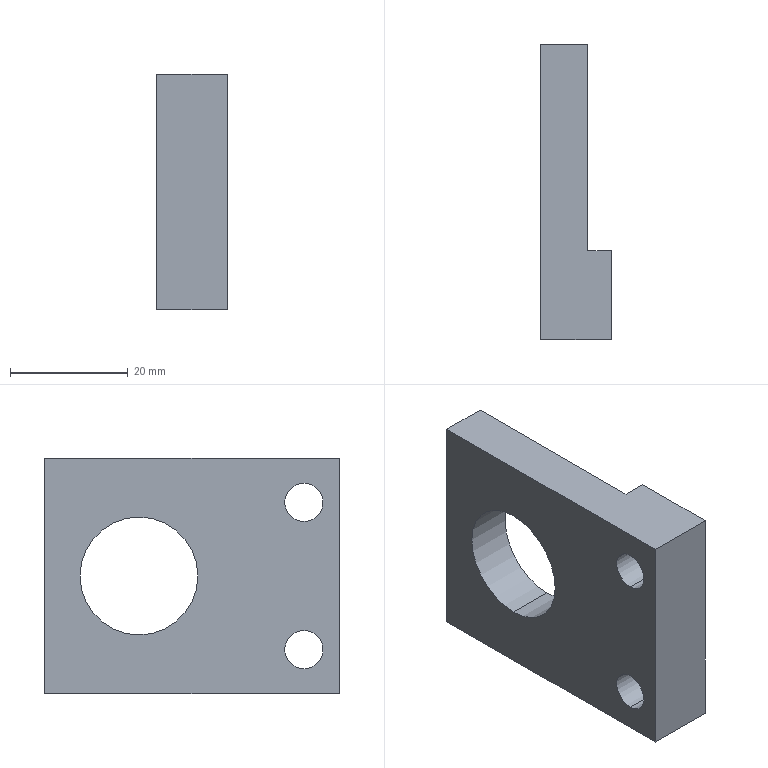Part | STEP file | cup material feed cylinder seat | 1 solid | 14 faces | box 12 x 50 x 40 mm | volume 15090 mm3 | plane 8 | cylinder 6 | commonest cylinder face diameters 6.5 x4 20 x2
STEP:
#1=CARTESIAN_POINT('',(0.,0.,0.));
#2=DIRECTION('',(0.,0.,1.));
#3=DIRECTION('',(1.,0.,0.));
#4=AXIS2_PLACEMENT_3D('',#1,#2,#3);
#5=CARTESIAN_POINT('',(0.,34.,-10.));
#6=VERTEX_POINT('',#5);
#7=CARTESIAN_POINT('',(8.,34.,-10.));
#8=VERTEX_POINT('',#7);
#9=CARTESIAN_POINT('',(8.,34.,-10.));
#10=DIRECTION('',(1.,0.,0.));
#11=VECTOR('',#10,1.);
#12=LINE('',#9,#11);
#13=CARTESIAN_POINT('',(8.,34.,0.));
#14=DIRECTION('',(1.,0.,0.));
#15=DIRECTION('',(0.,0.,-1.));
#16=AXIS2_PLACEMENT_3D('',#13,#14,#15);
#17=CYLINDRICAL_SURFACE('',#16,10.);
#18=CARTESIAN_POINT('',(6.283,0.));
#19=DIRECTION('',(0.,1.));
#20=VECTOR('',#19,1.);
#21=LINE('',#18,#20);
#22=(GEOMETRIC_REPRESENTATION_CONTEXT(2)PARAMETRIC_REPRESENTATION_CONTEXT()REPRESENTATION_CONTEXT('',''));
#23=DEFINITIONAL_REPRESENTATION('',(#21),#22);
#24=PCURVE('',#17,#23);
#25=CARTESIAN_POINT('',(8.,34.,0.));
#26=DIRECTION('',(1.,0.,0.));
#27=DIRECTION('',(0.,0.,-1.));
#28=AXIS2_PLACEMENT_3D('',#25,#26,#27);
#29=CYLINDRICAL_SURFACE('',#28,10.);
#30=CARTESIAN_POINT('',(0.,0.));
#31=DIRECTION('',(0.,1.));
#32=VECTOR('',#31,1.);
#33=LINE('',#30,#32);
#34=(GEOMETRIC_REPRESENTATION_CONTEXT(2)PARAMETRIC_REPRESENTATION_CONTEXT()REPRESENTATION_CONTEXT('',''));
#35=DEFINITIONAL_REPRESENTATION('',(#33),#34);
#36=PCURVE('',#29,#35);
#37=SURFACE_CURVE('',#12,(#24,#36),.PCURVE_S1.);
#38=EDGE_CURVE('',#6,#8,#37,.T.);
#39=ORIENTED_EDGE('',*,*,#38,.T.);
#40=CARTESIAN_POINT('',(8.,34.,10.));
#41=VERTEX_POINT('',#40);
#42=CARTESIAN_POINT('',(8.,34.,0.));
#43=DIRECTION('',(1.,0.,0.));
#44=DIRECTION('',(0.,0.,-1.));
#45=AXIS2_PLACEMENT_3D('',#42,#43,#44);
#46=CIRCLE('',#45,10.);
#47=CARTESIAN_POINT('',(0.,0.));
#48=DIRECTION('',(1.,0.));
#49=VECTOR('',#48,1.);
#50=LINE('',#47,#49);
#51=(GEOMETRIC_REPRESENTATION_CONTEXT(2)PARAMETRIC_REPRESENTATION_CONTEXT()REPRESENTATION_CONTEXT('',''));
#52=DEFINITIONAL_REPRESENTATION('',(#50),#51);
#53=PCURVE('',#17,#52);
#54=CARTESIAN_POINT('',(8.,50.,-20.));
#55=DIRECTION('',(1.,0.,0.));
#56=DIRECTION('',(0.,0.,-1.));
#57=AXIS2_PLACEMENT_3D('',#54,#55,#56);
#58=PLANE('',#57);
#59=CARTESIAN_POINT('',(-20.,-16.));
#60=DIRECTION('',(1.,0.));
#61=AXIS2_PLACEMENT_2D('',#59,#60);
#62=CIRCLE('',#61,10.);
#63=(GEOMETRIC_REPRESENTATION_CONTEXT(2)PARAMETRIC_REPRESENTATION_CONTEXT()REPRESENTATION_CONTEXT('',''));
#64=DEFINITIONAL_REPRESENTATION('',(#62),#63);
#65=PCURVE('',#58,#64);
#66=SURFACE_CURVE('',#46,(#53,#65),.PCURVE_S1.);
#67=EDGE_CURVE('',#41,#8,#66,.T.);
#68=ORIENTED_EDGE('',*,*,#67,.F.);
#69=CARTESIAN_POINT('',(0.,34.,10.));
#70=VERTEX_POINT('',#69);
#71=CARTESIAN_POINT('',(8.,34.,10.));
#72=DIRECTION('',(1.,0.,0.));
#73=VECTOR('',#72,1.);
#74=LINE('',#71,#73);
#75=CARTESIAN_POINT('',(3.142,0.));
#76=DIRECTION('',(0.,1.));
#77=VECTOR('',#76,1.);
#78=LINE('',#75,#77);
#79=(GEOMETRIC_REPRESENTATION_CONTEXT(2)PARAMETRIC_REPRESENTATION_CONTEXT()REPRESENTATION_CONTEXT('',''));
#80=DEFINITIONAL_REPRESENTATION('',(#78),#79);
#81=PCURVE('',#17,#80);
#82=CARTESIAN_POINT('',(3.142,0.));
#83=DIRECTION('',(0.,1.));
#84=VECTOR('',#83,1.);
#85=LINE('',#82,#84);
#86=(GEOMETRIC_REPRESENTATION_CONTEXT(2)PARAMETRIC_REPRESENTATION_CONTEXT()REPRESENTATION_CONTEXT('',''));
#87=DEFINITIONAL_REPRESENTATION('',(#85),#86);
#88=PCURVE('',#29,#87);
#89=SURFACE_CURVE('',#74,(#81,#88),.PCURVE_S1.);
#90=EDGE_CURVE('',#70,#41,#89,.T.);
#91=ORIENTED_EDGE('',*,*,#90,.F.);
#92=CARTESIAN_POINT('',(0.,34.,0.));
#93=DIRECTION('',(-1.,0.,0.));
#94=DIRECTION('',(0.,0.,1.));
#95=AXIS2_PLACEMENT_3D('',#92,#93,#94);
#96=CIRCLE('',#95,10.);
#97=CARTESIAN_POINT('',(9.425,-8.));
#98=DIRECTION('',(-1.,0.));
#99=VECTOR('',#98,1.);
#100=LINE('',#97,#99);
#101=(GEOMETRIC_REPRESENTATION_CONTEXT(2)PARAMETRIC_REPRESENTATION_CONTEXT()REPRESENTATION_CONTEXT('',''));
#102=DEFINITIONAL_REPRESENTATION('',(#100),#101);
#103=PCURVE('',#17,#102);
#104=CARTESIAN_POINT('',(0.,50.,-20.));
#105=DIRECTION('',(-1.,0.,0.));
#106=DIRECTION('',(0.,0.,1.));
#107=AXIS2_PLACEMENT_3D('',#104,#105,#106);
#108=PLANE('',#107);
#109=CARTESIAN_POINT('',(20.,-16.));
#110=DIRECTION('',(1.,0.));
#111=AXIS2_PLACEMENT_2D('',#109,#110);
#112=CIRCLE('',#111,10.);
#113=(GEOMETRIC_REPRESENTATION_CONTEXT(2)PARAMETRIC_REPRESENTATION_CONTEXT()REPRESENTATION_CONTEXT('',''));
#114=DEFINITIONAL_REPRESENTATION('',(#112),#113);
#115=PCURVE('',#108,#114);
#116=SURFACE_CURVE('',#96,(#103,#115),.PCURVE_S1.);
#117=EDGE_CURVE('',#6,#70,#116,.T.);
#118=ORIENTED_EDGE('',*,*,#117,.F.);
#119=EDGE_LOOP('',(#39,#68,#91,#118));
#120=FACE_BOUND('',#119,.F.);
#121=ADVANCED_FACE('',(#120),#17,.F.);
#122=CARTESIAN_POINT('',(0.,6.,9.25));
#123=VERTEX_POINT('',#122);
#124=CARTESIAN_POINT('',(12.,6.,9.25));
#125=VERTEX_POINT('',#124);
#126=CARTESIAN_POINT('',(12.,6.,9.25));
#127=DIRECTION('',(1.,0.,0.));
#128=VECTOR('',#127,1.);
#129=LINE('',#126,#128);
#130=CARTESIAN_POINT('',(12.,6.,12.5));
#131=DIRECTION('',(1.,0.,0.));
#132=DIRECTION('',(0.,0.,-1.));
#133=AXIS2_PLACEMENT_3D('',#130,#131,#132);
#134=CYLINDRICAL_SURFACE('',#133,3.25);
#135=CARTESIAN_POINT('',(6.283,0.));
#136=DIRECTION('',(0.,1.));
#137=VECTOR('',#136,1.);
#138=LINE('',#135,#137);
#139=(GEOMETRIC_REPRESENTATION_CONTEXT(2)PARAMETRIC_REPRESENTATION_CONTEXT()REPRESENTATION_CONTEXT('',''));
#140=DEFINITIONAL_REPRESENTATION('',(#138),#139);
#141=PCURVE('',#134,#140);
#142=CARTESIAN_POINT('',(12.,6.,12.5));
#143=DIRECTION('',(1.,0.,0.));
#144=DIRECTION('',(0.,0.,-1.));
#145=AXIS2_PLACEMENT_3D('',#142,#143,#144);
#146=CYLINDRICAL_SURFACE('',#145,3.25);
#147=CARTESIAN_POINT('',(0.,0.));
#148=DIRECTION('',(0.,1.));
#149=VECTOR('',#148,1.);
#150=LINE('',#147,#149);
#151=(GEOMETRIC_REPRESENTATION_CONTEXT(2)PARAMETRIC_REPRESENTATION_CONTEXT()REPRESENTATION_CONTEXT('',''));
#152=DEFINITIONAL_REPRESENTATION('',(#150),#151);
#153=PCURVE('',#146,#152);
#154=SURFACE_CURVE('',#129,(#141,#153),.PCURVE_S1.);
#155=EDGE_CURVE('',#123,#125,#154,.T.);
#156=ORIENTED_EDGE('',*,*,#155,.T.);
#157=CARTESIAN_POINT('',(12.,6.,15.75));
#158=VERTEX_POINT('',#157);
#159=CARTESIAN_POINT('',(12.,6.,12.5));
#160=DIRECTION('',(1.,0.,0.));
#161=DIRECTION('',(0.,0.,-1.));
#162=AXIS2_PLACEMENT_3D('',#159,#160,#161);
#163=CIRCLE('',#162,3.25);
#164=CARTESIAN_POINT('',(0.,0.));
#165=DIRECTION('',(1.,0.));
#166=VECTOR('',#165,1.);
#167=LINE('',#164,#166);
#168=(GEOMETRIC_REPRESENTATION_CONTEXT(2)PARAMETRIC_REPRESENTATION_CONTEXT()REPRESENTATION_CONTEXT('',''));
#169=DEFINITIONAL_REPRESENTATION('',(#167),#168);
#170=PCURVE('',#134,#169);
#171=CARTESIAN_POINT('',(12.,15.,-20.));
#172=DIRECTION('',(1.,0.,0.));
#173=DIRECTION('',(0.,0.,-1.));
#174=AXIS2_PLACEMENT_3D('',#171,#172,#173);
#175=PLANE('',#174);
#176=CARTESIAN_POINT('',(-32.5,-9.));
#177=DIRECTION('',(1.,0.));
#178=AXIS2_PLACEMENT_2D('',#176,#177);
#179=CIRCLE('',#178,3.25);
#180=(GEOMETRIC_REPRESENTATION_CONTEXT(2)PARAMETRIC_REPRESENTATION_CONTEXT()REPRESENTATION_CONTEXT('',''));
#181=DEFINITIONAL_REPRESENTATION('',(#179),#180);
#182=PCURVE('',#175,#181);
#183=SURFACE_CURVE('',#163,(#170,#182),.PCURVE_S1.);
#184=EDGE_CURVE('',#158,#125,#183,.T.);
#185=ORIENTED_EDGE('',*,*,#184,.F.);
#186=CARTESIAN_POINT('',(0.,6.,15.75));
#187=VERTEX_POINT('',#186);
#188=CARTESIAN_POINT('',(12.,6.,15.75));
#189=DIRECTION('',(1.,0.,0.));
#190=VECTOR('',#189,1.);
#191=LINE('',#188,#190);
#192=CARTESIAN_POINT('',(3.142,0.));
#193=DIRECTION('',(0.,1.));
#194=VECTOR('',#193,1.);
#195=LINE('',#192,#194);
#196=(GEOMETRIC_REPRESENTATION_CONTEXT(2)PARAMETRIC_REPRESENTATION_CONTEXT()REPRESENTATION_CONTEXT('',''));
#197=DEFINITIONAL_REPRESENTATION('',(#195),#196);
#198=PCURVE('',#134,#197);
#199=CARTESIAN_POINT('',(3.142,0.));
#200=DIRECTION('',(0.,1.));
#201=VECTOR('',#200,1.);
#202=LINE('',#199,#201);
#203=(GEOMETRIC_REPRESENTATION_CONTEXT(2)PARAMETRIC_REPRESENTATION_CONTEXT()REPRESENTATION_CONTEXT('',''));
#204=DEFINITIONAL_REPRESENTATION('',(#202),#203);
#205=PCURVE('',#146,#204);
#206=SURFACE_CURVE('',#191,(#198,#205),.PCURVE_S1.);
#207=EDGE_CURVE('',#187,#158,#206,.T.);
#208=ORIENTED_EDGE('',*,*,#207,.F.);
#209=CARTESIAN_POINT('',(0.,6.,12.5));
#210=DIRECTION('',(1.,0.,0.));
#211=DIRECTION('',(0.,0.,-1.));
#212=AXIS2_PLACEMENT_3D('',#209,#210,#211);
#213=CIRCLE('',#212,3.25);
#214=CARTESIAN_POINT('',(0.,-12.));
#215=DIRECTION('',(1.,0.));
#216=VECTOR('',#215,1.);
#217=LINE('',#214,#216);
#218=(GEOMETRIC_REPRESENTATION_CONTEXT(2)PARAMETRIC_REPRESENTATION_CONTEXT()REPRESENTATION_CONTEXT('',''));
#219=DEFINITIONAL_REPRESENTATION('',(#217),#218);
#220=PCURVE('',#134,#219);
#221=CARTESIAN_POINT('',(29.25,-44.));
#222=CARTESIAN_POINT('',(29.25,-38.371));
#223=CARTESIAN_POINT('',(34.125,-41.185));
#224=CARTESIAN_POINT('',(39.,-44.));
#225=CARTESIAN_POINT('',(34.125,-46.815));
#226=CARTESIAN_POINT('',(29.25,-49.629));
#227=CARTESIAN_POINT('',(29.25,-44.));
#228=(BOUNDED_CURVE()B_SPLINE_CURVE(2,(#221,#222,#223,#224,#225,#226,#227),.UNSPECIFIED.,.T.,.F.)B_SPLINE_CURVE_WITH_KNOTS((1,2,2,2,2,1),(-2.094,0.,2.094,4.189,6.283,8.378),.UNSPECIFIED.)CURVE()GEOMETRIC_REPRESENTATION_ITEM()RATIONAL_B_SPLINE_CURVE((1.,0.5,1.,0.5,1.,0.5,1.))REPRESENTATION_ITEM(''));
#229=(GEOMETRIC_REPRESENTATION_CONTEXT(2)PARAMETRIC_REPRESENTATION_CONTEXT()REPRESENTATION_CONTEXT('',''));
#230=DEFINITIONAL_REPRESENTATION('',(#228),#229);
#231=PCURVE('',#108,#230);
#232=SURFACE_CURVE('',#213,(#220,#231),.PCURVE_S1.);
#233=EDGE_CURVE('',#187,#123,#232,.T.);
#234=ORIENTED_EDGE('',*,*,#233,.T.);
#235=EDGE_LOOP('',(#156,#185,#208,#234));
#236=FACE_BOUND('',#235,.F.);
#237=ADVANCED_FACE('',(#236),#134,.F.);
#238=CARTESIAN_POINT('',(0.,6.,-15.75));
#239=VERTEX_POINT('',#238);
#240=CARTESIAN_POINT('',(12.,6.,-15.75));
#241=VERTEX_POINT('',#240);
#242=CARTESIAN_POINT('',(12.,6.,-15.75));
#243=DIRECTION('',(1.,0.,0.));
#244=VECTOR('',#243,1.);
#245=LINE('',#242,#244);
#246=CARTESIAN_POINT('',(12.,6.,-12.5));
#247=DIRECTION('',(1.,0.,0.));
#248=DIRECTION('',(0.,0.,-1.));
#249=AXIS2_PLACEMENT_3D('',#246,#247,#248);
#250=CYLINDRICAL_SURFACE('',#249,3.25);
#251=CARTESIAN_POINT('',(6.283,0.));
#252=DIRECTION('',(0.,1.));
#253=VECTOR('',#252,1.);
#254=LINE('',#251,#253);
#255=(GEOMETRIC_REPRESENTATION_CONTEXT(2)PARAMETRIC_REPRESENTATION_CONTEXT()REPRESENTATION_CONTEXT('',''));
#256=DEFINITIONAL_REPRESENTATION('',(#254),#255);
#257=PCURVE('',#250,#256);
#258=CARTESIAN_POINT('',(12.,6.,-12.5));
#259=DIRECTION('',(1.,0.,0.));
#260=DIRECTION('',(0.,0.,-1.));
#261=AXIS2_PLACEMENT_3D('',#258,#259,#260);
#262=CYLINDRICAL_SURFACE('',#261,3.25);
#263=CARTESIAN_POINT('',(0.,0.));
#264=DIRECTION('',(0.,1.));
#265=VECTOR('',#264,1.);
#266=LINE('',#263,#265);
#267=(GEOMETRIC_REPRESENTATION_CONTEXT(2)PARAMETRIC_REPRESENTATION_CONTEXT()REPRESENTATION_CONTEXT('',''));
#268=DEFINITIONAL_REPRESENTATION('',(#266),#267);
#269=PCURVE('',#262,#268);
#270=SURFACE_CURVE('',#245,(#257,#269),.PCURVE_S1.);
#271=EDGE_CURVE('',#239,#241,#270,.T.);
#272=ORIENTED_EDGE('',*,*,#271,.T.);
#273=CARTESIAN_POINT('',(12.,6.,-9.25));
#274=VERTEX_POINT('',#273);
#275=CARTESIAN_POINT('',(12.,6.,-12.5));
#276=DIRECTION('',(1.,0.,0.));
#277=DIRECTION('',(0.,0.,-1.));
#278=AXIS2_PLACEMENT_3D('',#275,#276,#277);
#279=CIRCLE('',#278,3.25);
#280=CARTESIAN_POINT('',(0.,0.));
#281=DIRECTION('',(1.,0.));
#282=VECTOR('',#281,1.);
#283=LINE('',#280,#282);
#284=(GEOMETRIC_REPRESENTATION_CONTEXT(2)PARAMETRIC_REPRESENTATION_CONTEXT()REPRESENTATION_CONTEXT('',''));
#285=DEFINITIONAL_REPRESENTATION('',(#283),#284);
#286=PCURVE('',#250,#285);
#287=CARTESIAN_POINT('',(-7.5,-9.));
#288=DIRECTION('',(1.,0.));
#289=AXIS2_PLACEMENT_2D('',#287,#288);
#290=CIRCLE('',#289,3.25);
#291=(GEOMETRIC_REPRESENTATION_CONTEXT(2)PARAMETRIC_REPRESENTATION_CONTEXT()REPRESENTATION_CONTEXT('',''));
#292=DEFINITIONAL_REPRESENTATION('',(#290),#291);
#293=PCURVE('',#175,#292);
#294=SURFACE_CURVE('',#279,(#286,#293),.PCURVE_S1.);
#295=EDGE_CURVE('',#274,#241,#294,.T.);
#296=ORIENTED_EDGE('',*,*,#295,.F.);
#297=CARTESIAN_POINT('',(0.,6.,-9.25));
#298=VERTEX_POINT('',#297);
#299=CARTESIAN_POINT('',(12.,6.,-9.25));
#300=DIRECTION('',(1.,0.,0.));
#301=VECTOR('',#300,1.);
#302=LINE('',#299,#301);
#303=CARTESIAN_POINT('',(3.142,0.));
#304=DIRECTION('',(0.,1.));
#305=VECTOR('',#304,1.);
#306=LINE('',#303,#305);
#307=(GEOMETRIC_REPRESENTATION_CONTEXT(2)PARAMETRIC_REPRESENTATION_CONTEXT()REPRESENTATION_CONTEXT('',''));
#308=DEFINITIONAL_REPRESENTATION('',(#306),#307);
#309=PCURVE('',#250,#308);
#310=CARTESIAN_POINT('',(3.142,0.));
#311=DIRECTION('',(0.,1.));
#312=VECTOR('',#311,1.);
#313=LINE('',#310,#312);
#314=(GEOMETRIC_REPRESENTATION_CONTEXT(2)PARAMETRIC_REPRESENTATION_CONTEXT()REPRESENTATION_CONTEXT('',''));
#315=DEFINITIONAL_REPRESENTATION('',(#313),#314);
#316=PCURVE('',#262,#315);
#317=SURFACE_CURVE('',#302,(#309,#316),.PCURVE_S1.);
#318=EDGE_CURVE('',#298,#274,#317,.T.);
#319=ORIENTED_EDGE('',*,*,#318,.F.);
#320=CARTESIAN_POINT('',(0.,6.,-12.5));
#321=DIRECTION('',(1.,0.,0.));
#322=DIRECTION('',(0.,0.,-1.));
#323=AXIS2_PLACEMENT_3D('',#320,#321,#322);
#324=CIRCLE('',#323,3.25);
#325=CARTESIAN_POINT('',(0.,-12.));
#326=DIRECTION('',(1.,0.));
#327=VECTOR('',#326,1.);
#328=LINE('',#325,#327);
#329=(GEOMETRIC_REPRESENTATION_CONTEXT(2)PARAMETRIC_REPRESENTATION_CONTEXT()REPRESENTATION_CONTEXT('',''));
#330=DEFINITIONAL_REPRESENTATION('',(#328),#329);
#331=PCURVE('',#250,#330);
#332=CARTESIAN_POINT('',(4.25,-44.));
#333=CARTESIAN_POINT('',(4.25,-38.371));
#334=CARTESIAN_POINT('',(9.125,-41.185));
#335=CARTESIAN_POINT('',(14.,-44.));
#336=CARTESIAN_POINT('',(9.125,-46.815));
#337=CARTESIAN_POINT('',(4.25,-49.629));
#338=CARTESIAN_POINT('',(4.25,-44.));
#339=(BOUNDED_CURVE()B_SPLINE_CURVE(2,(#332,#333,#334,#335,#336,#337,#338),.UNSPECIFIED.,.T.,.F.)B_SPLINE_CURVE_WITH_KNOTS((1,2,2,2,2,1),(-2.094,0.,2.094,4.189,6.283,8.378),.UNSPECIFIED.)CURVE()GEOMETRIC_REPRESENTATION_ITEM()RATIONAL_B_SPLINE_CURVE((1.,0.5,1.,0.5,1.,0.5,1.))REPRESENTATION_ITEM(''));
#340=(GEOMETRIC_REPRESENTATION_CONTEXT(2)PARAMETRIC_REPRESENTATION_CONTEXT()REPRESENTATION_CONTEXT('',''));
#341=DEFINITIONAL_REPRESENTATION('',(#339),#340);
#342=PCURVE('',#108,#341);
#343=SURFACE_CURVE('',#324,(#331,#342),.PCURVE_S1.);
#344=EDGE_CURVE('',#298,#239,#343,.T.);
#345=ORIENTED_EDGE('',*,*,#344,.T.);
#346=EDGE_LOOP('',(#272,#296,#319,#345));
#347=FACE_BOUND('',#346,.F.);
#348=ADVANCED_FACE('',(#347),#250,.F.);
#349=ORIENTED_EDGE('',*,*,#117,.F.);
#350=CARTESIAN_POINT('',(0.,34.,0.));
#351=DIRECTION('',(-1.,0.,0.));
#352=DIRECTION('',(0.,0.,1.));
#353=AXIS2_PLACEMENT_3D('',#350,#351,#352);
#354=CIRCLE('',#353,10.);
#355=CARTESIAN_POINT('',(20.,-16.));
#356=DIRECTION('',(1.,0.));
#357=AXIS2_PLACEMENT_2D('',#355,#356);
#358=CIRCLE('',#357,10.);
#359=(GEOMETRIC_REPRESENTATION_CONTEXT(2)PARAMETRIC_REPRESENTATION_CONTEXT()REPRESENTATION_CONTEXT('',''));
#360=DEFINITIONAL_REPRESENTATION('',(#358),#359);
#361=PCURVE('',#108,#360);
#362=CARTESIAN_POINT('',(3.142,-8.));
#363=DIRECTION('',(-1.,0.));
#364=VECTOR('',#363,1.);
#365=LINE('',#362,#364);
#366=(GEOMETRIC_REPRESENTATION_CONTEXT(2)PARAMETRIC_REPRESENTATION_CONTEXT()REPRESENTATION_CONTEXT('',''));
#367=DEFINITIONAL_REPRESENTATION('',(#365),#366);
#368=PCURVE('',#29,#367);
#369=SURFACE_CURVE('',#354,(#361,#368),.PCURVE_S1.);
#370=EDGE_CURVE('',#70,#6,#369,.T.);
#371=ORIENTED_EDGE('',*,*,#370,.F.);
#372=EDGE_LOOP('',(#349,#371));
#373=FACE_BOUND('',#372,.T.);
#374=CARTESIAN_POINT('',(0.,6.,12.5));
#375=DIRECTION('',(1.,0.,0.));
#376=DIRECTION('',(0.,0.,-1.));
#377=AXIS2_PLACEMENT_3D('',#374,#375,#376);
#378=CIRCLE('',#377,3.25);
#379=CARTESIAN_POINT('',(29.25,-44.));
#380=CARTESIAN_POINT('',(29.25,-38.371));
#381=CARTESIAN_POINT('',(34.125,-41.185));
#382=CARTESIAN_POINT('',(39.,-44.));
#383=CARTESIAN_POINT('',(34.125,-46.815));
#384=CARTESIAN_POINT('',(29.25,-49.629));
#385=CARTESIAN_POINT('',(29.25,-44.));
#386=(BOUNDED_CURVE()B_SPLINE_CURVE(2,(#379,#380,#381,#382,#383,#384,#385),.UNSPECIFIED.,.T.,.F.)B_SPLINE_CURVE_WITH_KNOTS((1,2,2,2,2,1),(-2.094,0.,2.094,4.189,6.283,8.378),.UNSPECIFIED.)CURVE()GEOMETRIC_REPRESENTATION_ITEM()RATIONAL_B_SPLINE_CURVE((1.,0.5,1.,0.5,1.,0.5,1.))REPRESENTATION_ITEM(''));
#387=(GEOMETRIC_REPRESENTATION_CONTEXT(2)PARAMETRIC_REPRESENTATION_CONTEXT()REPRESENTATION_CONTEXT('',''));
#388=DEFINITIONAL_REPRESENTATION('',(#386),#387);
#389=PCURVE('',#108,#388);
#390=CARTESIAN_POINT('',(0.,-12.));
#391=DIRECTION('',(1.,0.));
#392=VECTOR('',#391,1.);
#393=LINE('',#390,#392);
#394=(GEOMETRIC_REPRESENTATION_CONTEXT(2)PARAMETRIC_REPRESENTATION_CONTEXT()REPRESENTATION_CONTEXT('',''));
#395=DEFINITIONAL_REPRESENTATION('',(#393),#394);
#396=PCURVE('',#146,#395);
#397=SURFACE_CURVE('',#378,(#389,#396),.PCURVE_S1.);
#398=EDGE_CURVE('',#123,#187,#397,.T.);
#399=ORIENTED_EDGE('',*,*,#398,.T.);
#400=ORIENTED_EDGE('',*,*,#233,.T.);
#401=EDGE_LOOP('',(#399,#400));
#402=FACE_BOUND('',#401,.T.);
#403=CARTESIAN_POINT('',(0.,6.,-12.5));
#404=DIRECTION('',(1.,0.,0.));
#405=DIRECTION('',(0.,0.,-1.));
#406=AXIS2_PLACEMENT_3D('',#403,#404,#405);
#407=CIRCLE('',#406,3.25);
#408=CARTESIAN_POINT('',(4.25,-44.));
#409=CARTESIAN_POINT('',(4.25,-38.371));
#410=CARTESIAN_POINT('',(9.125,-41.185));
#411=CARTESIAN_POINT('',(14.,-44.));
#412=CARTESIAN_POINT('',(9.125,-46.815));
#413=CARTESIAN_POINT('',(4.25,-49.629));
#414=CARTESIAN_POINT('',(4.25,-44.));
#415=(BOUNDED_CURVE()B_SPLINE_CURVE(2,(#408,#409,#410,#411,#412,#413,#414),.UNSPECIFIED.,.T.,.F.)B_SPLINE_CURVE_WITH_KNOTS((1,2,2,2,2,1),(-2.094,0.,2.094,4.189,6.283,8.378),.UNSPECIFIED.)CURVE()GEOMETRIC_REPRESENTATION_ITEM()RATIONAL_B_SPLINE_CURVE((1.,0.5,1.,0.5,1.,0.5,1.))REPRESENTATION_ITEM(''));
#416=(GEOMETRIC_REPRESENTATION_CONTEXT(2)PARAMETRIC_REPRESENTATION_CONTEXT()REPRESENTATION_CONTEXT('',''));
#417=DEFINITIONAL_REPRESENTATION('',(#415),#416);
#418=PCURVE('',#108,#417);
#419=CARTESIAN_POINT('',(0.,-12.));
#420=DIRECTION('',(1.,0.));
#421=VECTOR('',#420,1.);
#422=LINE('',#419,#421);
#423=(GEOMETRIC_REPRESENTATION_CONTEXT(2)PARAMETRIC_REPRESENTATION_CONTEXT()REPRESENTATION_CONTEXT('',''));
#424=DEFINITIONAL_REPRESENTATION('',(#422),#423);
#425=PCURVE('',#262,#424);
#426=SURFACE_CURVE('',#407,(#418,#425),.PCURVE_S1.);
#427=EDGE_CURVE('',#239,#298,#426,.T.);
#428=ORIENTED_EDGE('',*,*,#427,.T.);
#429=ORIENTED_EDGE('',*,*,#344,.T.);
#430=EDGE_LOOP('',(#428,#429));
#431=FACE_BOUND('',#430,.T.);
#432=CARTESIAN_POINT('',(0.,0.,-20.));
#433=VERTEX_POINT('',#432);
#434=CARTESIAN_POINT('',(0.,0.,20.));
#435=VERTEX_POINT('',#434);
#436=CARTESIAN_POINT('',(0.,0.,-20.));
#437=DIRECTION('',(0.,0.,1.));
#438=VECTOR('',#437,1.);
#439=LINE('',#436,#438);
#440=CARTESIAN_POINT('',(0.,-50.));
#441=DIRECTION('',(1.,0.));
#442=VECTOR('',#441,1.);
#443=LINE('',#440,#442);
#444=(GEOMETRIC_REPRESENTATION_CONTEXT(2)PARAMETRIC_REPRESENTATION_CONTEXT()REPRESENTATION_CONTEXT('',''));
#445=DEFINITIONAL_REPRESENTATION('',(#443),#444);
#446=PCURVE('',#108,#445);
#447=CARTESIAN_POINT('',(0.,0.,-20.));
#448=DIRECTION('',(0.,-1.,0.));
#449=DIRECTION('',(0.,0.,-1.));
#450=AXIS2_PLACEMENT_3D('',#447,#448,#449);
#451=PLANE('',#450);
#452=CARTESIAN_POINT('',(0.,0.));
#453=DIRECTION('',(-1.,0.));
#454=VECTOR('',#453,1.);
#455=LINE('',#452,#454);
#456=(GEOMETRIC_REPRESENTATION_CONTEXT(2)PARAMETRIC_REPRESENTATION_CONTEXT()REPRESENTATION_CONTEXT('',''));
#457=DEFINITIONAL_REPRESENTATION('',(#455),#456);
#458=PCURVE('',#451,#457);
#459=SURFACE_CURVE('',#439,(#446,#458),.PCURVE_S1.);
#460=EDGE_CURVE('',#433,#435,#459,.T.);
#461=ORIENTED_EDGE('',*,*,#460,.T.);
#462=CARTESIAN_POINT('',(0.,50.,20.));
#463=VERTEX_POINT('',#462);
#464=CARTESIAN_POINT('',(0.,50.,20.));
#465=DIRECTION('',(0.,-1.,0.));
#466=VECTOR('',#465,1.);
#467=LINE('',#464,#466);
#468=CARTESIAN_POINT('',(40.,0.));
#469=DIRECTION('',(0.,-1.));
#470=VECTOR('',#469,1.);
#471=LINE('',#468,#470);
#472=(GEOMETRIC_REPRESENTATION_CONTEXT(2)PARAMETRIC_REPRESENTATION_CONTEXT()REPRESENTATION_CONTEXT('',''));
#473=DEFINITIONAL_REPRESENTATION('',(#471),#472);
#474=PCURVE('',#108,#473);
#475=CARTESIAN_POINT('',(0.,0.,20.));
#476=DIRECTION('',(0.,0.,1.));
#477=DIRECTION('',(1.,0.,0.));
#478=AXIS2_PLACEMENT_3D('',#475,#476,#477);
#479=PLANE('',#478);
#480=CARTESIAN_POINT('',(0.,50.));
#481=DIRECTION('',(0.,-1.));
#482=VECTOR('',#481,1.);
#483=LINE('',#480,#482);
#484=(GEOMETRIC_REPRESENTATION_CONTEXT(2)PARAMETRIC_REPRESENTATION_CONTEXT()REPRESENTATION_CONTEXT('',''));
#485=DEFINITIONAL_REPRESENTATION('',(#483),#484);
#486=PCURVE('',#479,#485);
#487=SURFACE_CURVE('',#467,(#474,#486),.PCURVE_S1.);
#488=EDGE_CURVE('',#463,#435,#487,.T.);
#489=ORIENTED_EDGE('',*,*,#488,.F.);
#490=CARTESIAN_POINT('',(0.,50.,-20.));
#491=VERTEX_POINT('',#490);
#492=CARTESIAN_POINT('',(0.,50.,-20.));
#493=DIRECTION('',(0.,0.,1.));
#494=VECTOR('',#493,1.);
#495=LINE('',#492,#494);
#496=CARTESIAN_POINT('',(0.,0.));
#497=DIRECTION('',(1.,0.));
#498=VECTOR('',#497,1.);
#499=LINE('',#496,#498);
#500=(GEOMETRIC_REPRESENTATION_CONTEXT(2)PARAMETRIC_REPRESENTATION_CONTEXT()REPRESENTATION_CONTEXT('',''));
#501=DEFINITIONAL_REPRESENTATION('',(#499),#500);
#502=PCURVE('',#108,#501);
#503=CARTESIAN_POINT('',(0.,50.,-20.));
#504=DIRECTION('',(0.,1.,0.));
#505=DIRECTION('',(0.,0.,1.));
#506=AXIS2_PLACEMENT_3D('',#503,#504,#505);
#507=PLANE('',#506);
#508=CARTESIAN_POINT('',(0.,0.));
#509=DIRECTION('',(1.,0.));
#510=VECTOR('',#509,1.);
#511=LINE('',#508,#510);
#512=(GEOMETRIC_REPRESENTATION_CONTEXT(2)PARAMETRIC_REPRESENTATION_CONTEXT()REPRESENTATION_CONTEXT('',''));
#513=DEFINITIONAL_REPRESENTATION('',(#511),#512);
#514=PCURVE('',#507,#513);
#515=SURFACE_CURVE('',#495,(#502,#514),.PCURVE_S1.);
#516=EDGE_CURVE('',#491,#463,#515,.T.);
#517=ORIENTED_EDGE('',*,*,#516,.F.);
#518=CARTESIAN_POINT('',(0.,50.,-20.));
#519=DIRECTION('',(0.,-1.,0.));
#520=VECTOR('',#519,1.);
#521=LINE('',#518,#520);
#522=CARTESIAN_POINT('',(0.,0.));
#523=DIRECTION('',(0.,-1.));
#524=VECTOR('',#523,1.);
#525=LINE('',#522,#524);
#526=(GEOMETRIC_REPRESENTATION_CONTEXT(2)PARAMETRIC_REPRESENTATION_CONTEXT()REPRESENTATION_CONTEXT('',''));
#527=DEFINITIONAL_REPRESENTATION('',(#525),#526);
#528=PCURVE('',#108,#527);
#529=CARTESIAN_POINT('',(0.,0.,-20.));
#530=DIRECTION('',(0.,0.,1.));
#531=DIRECTION('',(1.,0.,0.));
#532=AXIS2_PLACEMENT_3D('',#529,#530,#531);
#533=PLANE('',#532);
#534=CARTESIAN_POINT('',(0.,50.));
#535=DIRECTION('',(0.,-1.));
#536=VECTOR('',#535,1.);
#537=LINE('',#534,#536);
#538=(GEOMETRIC_REPRESENTATION_CONTEXT(2)PARAMETRIC_REPRESENTATION_CONTEXT()REPRESENTATION_CONTEXT('',''));
#539=DEFINITIONAL_REPRESENTATION('',(#537),#538);
#540=PCURVE('',#533,#539);
#541=SURFACE_CURVE('',#521,(#528,#540),.PCURVE_S1.);
#542=EDGE_CURVE('',#491,#433,#541,.T.);
#543=ORIENTED_EDGE('',*,*,#542,.T.);
#544=EDGE_LOOP('',(#461,#489,#517,#543));
#545=FACE_BOUND('',#544,.T.);
#546=ADVANCED_FACE('',(#373,#402,#431,#545),#108,.T.);
#547=ORIENTED_EDGE('',*,*,#516,.T.);
#548=CARTESIAN_POINT('',(8.,50.,20.));
#549=VERTEX_POINT('',#548);
#550=CARTESIAN_POINT('',(0.,50.,20.));
#551=DIRECTION('',(-1.,0.,0.));
#552=VECTOR('',#551,1.);
#553=LINE('',#550,#552);
#554=CARTESIAN_POINT('',(40.,0.));
#555=DIRECTION('',(0.,-1.));
#556=VECTOR('',#555,1.);
#557=LINE('',#554,#556);
#558=(GEOMETRIC_REPRESENTATION_CONTEXT(2)PARAMETRIC_REPRESENTATION_CONTEXT()REPRESENTATION_CONTEXT('',''));
#559=DEFINITIONAL_REPRESENTATION('',(#557),#558);
#560=PCURVE('',#507,#559);
#561=CARTESIAN_POINT('',(0.,50.));
#562=DIRECTION('',(-1.,0.));
#563=VECTOR('',#562,1.);
#564=LINE('',#561,#563);
#565=(GEOMETRIC_REPRESENTATION_CONTEXT(2)PARAMETRIC_REPRESENTATION_CONTEXT()REPRESENTATION_CONTEXT('',''));
#566=DEFINITIONAL_REPRESENTATION('',(#564),#565);
#567=PCURVE('',#479,#566);
#568=SURFACE_CURVE('',#553,(#560,#567),.PCURVE_S1.);
#569=EDGE_CURVE('',#549,#463,#568,.T.);
#570=ORIENTED_EDGE('',*,*,#569,.F.);
#571=CARTESIAN_POINT('',(8.,50.,-20.));
#572=VERTEX_POINT('',#571);
#573=CARTESIAN_POINT('',(8.,50.,-20.));
#574=DIRECTION('',(0.,0.,1.));
#575=VECTOR('',#574,1.);
#576=LINE('',#573,#575);
#577=CARTESIAN_POINT('',(0.,8.));
#578=DIRECTION('',(1.,0.));
#579=VECTOR('',#578,1.);
#580=LINE('',#577,#579);
#581=(GEOMETRIC_REPRESENTATION_CONTEXT(2)PARAMETRIC_REPRESENTATION_CONTEXT()REPRESENTATION_CONTEXT('',''));
#582=DEFINITIONAL_REPRESENTATION('',(#580),#581);
#583=PCURVE('',#507,#582);
#584=CARTESIAN_POINT('',(0.,0.));
#585=DIRECTION('',(-1.,0.));
#586=VECTOR('',#585,1.);
#587=LINE('',#584,#586);
#588=(GEOMETRIC_REPRESENTATION_CONTEXT(2)PARAMETRIC_REPRESENTATION_CONTEXT()REPRESENTATION_CONTEXT('',''));
#589=DEFINITIONAL_REPRESENTATION('',(#587),#588);
#590=PCURVE('',#58,#589);
#591=SURFACE_CURVE('',#576,(#583,#590),.PCURVE_S1.);
#592=EDGE_CURVE('',#572,#549,#591,.T.);
#593=ORIENTED_EDGE('',*,*,#592,.F.);
#594=CARTESIAN_POINT('',(0.,50.,-20.));
#595=DIRECTION('',(-1.,0.,0.));
#596=VECTOR('',#595,1.);
#597=LINE('',#594,#596);
#598=CARTESIAN_POINT('',(0.,0.));
#599=DIRECTION('',(0.,-1.));
#600=VECTOR('',#599,1.);
#601=LINE('',#598,#600);
#602=(GEOMETRIC_REPRESENTATION_CONTEXT(2)PARAMETRIC_REPRESENTATION_CONTEXT()REPRESENTATION_CONTEXT('',''));
#603=DEFINITIONAL_REPRESENTATION('',(#601),#602);
#604=PCURVE('',#507,#603);
#605=CARTESIAN_POINT('',(0.,50.));
#606=DIRECTION('',(-1.,0.));
#607=VECTOR('',#606,1.);
#608=LINE('',#605,#607);
#609=(GEOMETRIC_REPRESENTATION_CONTEXT(2)PARAMETRIC_REPRESENTATION_CONTEXT()REPRESENTATION_CONTEXT('',''));
#610=DEFINITIONAL_REPRESENTATION('',(#608),#609);
#611=PCURVE('',#533,#610);
#612=SURFACE_CURVE('',#597,(#604,#611),.PCURVE_S1.);
#613=EDGE_CURVE('',#572,#491,#612,.T.);
#614=ORIENTED_EDGE('',*,*,#613,.T.);
#615=EDGE_LOOP('',(#547,#570,#593,#614));
#616=FACE_BOUND('',#615,.T.);
#617=ADVANCED_FACE('',(#616),#507,.T.);
#618=CARTESIAN_POINT('',(8.,34.,0.));
#619=DIRECTION('',(1.,0.,0.));
#620=DIRECTION('',(0.,0.,-1.));
#621=AXIS2_PLACEMENT_3D('',#618,#619,#620);
#622=CIRCLE('',#621,10.);
#623=CARTESIAN_POINT('',(-20.,-16.));
#624=DIRECTION('',(1.,0.));
#625=AXIS2_PLACEMENT_2D('',#623,#624);
#626=CIRCLE('',#625,10.);
#627=(GEOMETRIC_REPRESENTATION_CONTEXT(2)PARAMETRIC_REPRESENTATION_CONTEXT()REPRESENTATION_CONTEXT('',''));
#628=DEFINITIONAL_REPRESENTATION('',(#626),#627);
#629=PCURVE('',#58,#628);
#630=CARTESIAN_POINT('',(0.,0.));
#631=DIRECTION('',(1.,0.));
#632=VECTOR('',#631,1.);
#633=LINE('',#630,#632);
#634=(GEOMETRIC_REPRESENTATION_CONTEXT(2)PARAMETRIC_REPRESENTATION_CONTEXT()REPRESENTATION_CONTEXT('',''));
#635=DEFINITIONAL_REPRESENTATION('',(#633),#634);
#636=PCURVE('',#29,#635);
#637=SURFACE_CURVE('',#622,(#629,#636),.PCURVE_S1.);
#638=EDGE_CURVE('',#8,#41,#637,.T.);
#639=ORIENTED_EDGE('',*,*,#638,.F.);
#640=ORIENTED_EDGE('',*,*,#67,.F.);
#641=EDGE_LOOP('',(#639,#640));
#642=FACE_BOUND('',#641,.T.);
#643=ORIENTED_EDGE('',*,*,#592,.T.);
#644=CARTESIAN_POINT('',(8.,15.,20.));
#645=VERTEX_POINT('',#644);
#646=CARTESIAN_POINT('',(8.,50.,20.));
#647=DIRECTION('',(0.,1.,0.));
#648=VECTOR('',#647,1.);
#649=LINE('',#646,#648);
#650=CARTESIAN_POINT('',(-40.,0.));
#651=DIRECTION('',(0.,1.));
#652=VECTOR('',#651,1.);
#653=LINE('',#650,#652);
#654=(GEOMETRIC_REPRESENTATION_CONTEXT(2)PARAMETRIC_REPRESENTATION_CONTEXT()REPRESENTATION_CONTEXT('',''));
#655=DEFINITIONAL_REPRESENTATION('',(#653),#654);
#656=PCURVE('',#58,#655);
#657=CARTESIAN_POINT('',(8.,50.));
#658=DIRECTION('',(0.,1.));
#659=VECTOR('',#658,1.);
#660=LINE('',#657,#659);
#661=(GEOMETRIC_REPRESENTATION_CONTEXT(2)PARAMETRIC_REPRESENTATION_CONTEXT()REPRESENTATION_CONTEXT('',''));
#662=DEFINITIONAL_REPRESENTATION('',(#660),#661);
#663=PCURVE('',#479,#662);
#664=SURFACE_CURVE('',#649,(#656,#663),.PCURVE_S1.);
#665=EDGE_CURVE('',#645,#549,#664,.T.);
#666=ORIENTED_EDGE('',*,*,#665,.F.);
#667=CARTESIAN_POINT('',(8.,15.,-20.));
#668=VERTEX_POINT('',#667);
#669=CARTESIAN_POINT('',(8.,15.,-20.));
#670=DIRECTION('',(0.,0.,1.));
#671=VECTOR('',#670,1.);
#672=LINE('',#669,#671);
#673=CARTESIAN_POINT('',(0.,-35.));
#674=DIRECTION('',(-1.,0.));
#675=VECTOR('',#674,1.);
#676=LINE('',#673,#675);
#677=(GEOMETRIC_REPRESENTATION_CONTEXT(2)PARAMETRIC_REPRESENTATION_CONTEXT()REPRESENTATION_CONTEXT('',''));
#678=DEFINITIONAL_REPRESENTATION('',(#676),#677);
#679=PCURVE('',#58,#678);
#680=CARTESIAN_POINT('',(8.,15.,-20.));
#681=DIRECTION('',(0.,1.,0.));
#682=DIRECTION('',(0.,0.,1.));
#683=AXIS2_PLACEMENT_3D('',#680,#681,#682);
#684=PLANE('',#683);
#685=CARTESIAN_POINT('',(0.,0.));
#686=DIRECTION('',(1.,0.));
#687=VECTOR('',#686,1.);
#688=LINE('',#685,#687);
#689=(GEOMETRIC_REPRESENTATION_CONTEXT(2)PARAMETRIC_REPRESENTATION_CONTEXT()REPRESENTATION_CONTEXT('',''));
#690=DEFINITIONAL_REPRESENTATION('',(#688),#689);
#691=PCURVE('',#684,#690);
#692=SURFACE_CURVE('',#672,(#679,#691),.PCURVE_S1.);
#693=EDGE_CURVE('',#668,#645,#692,.T.);
#694=ORIENTED_EDGE('',*,*,#693,.F.);
#695=CARTESIAN_POINT('',(8.,50.,-20.));
#696=DIRECTION('',(0.,1.,0.));
#697=VECTOR('',#696,1.);
#698=LINE('',#695,#697);
#699=CARTESIAN_POINT('',(0.,0.));
#700=DIRECTION('',(0.,1.));
#701=VECTOR('',#700,1.);
#702=LINE('',#699,#701);
#703=(GEOMETRIC_REPRESENTATION_CONTEXT(2)PARAMETRIC_REPRESENTATION_CONTEXT()REPRESENTATION_CONTEXT('',''));
#704=DEFINITIONAL_REPRESENTATION('',(#702),#703);
#705=PCURVE('',#58,#704);
#706=CARTESIAN_POINT('',(8.,50.));
#707=DIRECTION('',(0.,1.));
#708=VECTOR('',#707,1.);
#709=LINE('',#706,#708);
#710=(GEOMETRIC_REPRESENTATION_CONTEXT(2)PARAMETRIC_REPRESENTATION_CONTEXT()REPRESENTATION_CONTEXT('',''));
#711=DEFINITIONAL_REPRESENTATION('',(#709),#710);
#712=PCURVE('',#533,#711);
#713=SURFACE_CURVE('',#698,(#705,#712),.PCURVE_S1.);
#714=EDGE_CURVE('',#668,#572,#713,.T.);
#715=ORIENTED_EDGE('',*,*,#714,.T.);
#716=EDGE_LOOP('',(#643,#666,#694,#715));
#717=FACE_BOUND('',#716,.T.);
#718=ADVANCED_FACE('',(#642,#717),#58,.T.);
#719=ORIENTED_EDGE('',*,*,#693,.T.);
#720=CARTESIAN_POINT('',(12.,15.,20.));
#721=VERTEX_POINT('',#720);
#722=CARTESIAN_POINT('',(8.,15.,20.));
#723=DIRECTION('',(-1.,0.,0.));
#724=VECTOR('',#723,1.);
#725=LINE('',#722,#724);
#726=CARTESIAN_POINT('',(40.,0.));
#727=DIRECTION('',(0.,-1.));
#728=VECTOR('',#727,1.);
#729=LINE('',#726,#728);
#730=(GEOMETRIC_REPRESENTATION_CONTEXT(2)PARAMETRIC_REPRESENTATION_CONTEXT()REPRESENTATION_CONTEXT('',''));
#731=DEFINITIONAL_REPRESENTATION('',(#729),#730);
#732=PCURVE('',#684,#731);
#733=CARTESIAN_POINT('',(8.,15.));
#734=DIRECTION('',(-1.,0.));
#735=VECTOR('',#734,1.);
#736=LINE('',#733,#735);
#737=(GEOMETRIC_REPRESENTATION_CONTEXT(2)PARAMETRIC_REPRESENTATION_CONTEXT()REPRESENTATION_CONTEXT('',''));
#738=DEFINITIONAL_REPRESENTATION('',(#736),#737);
#739=PCURVE('',#479,#738);
#740=SURFACE_CURVE('',#725,(#732,#739),.PCURVE_S1.);
#741=EDGE_CURVE('',#721,#645,#740,.T.);
#742=ORIENTED_EDGE('',*,*,#741,.F.);
#743=CARTESIAN_POINT('',(12.,15.,-20.));
#744=VERTEX_POINT('',#743);
#745=CARTESIAN_POINT('',(12.,15.,-20.));
#746=DIRECTION('',(0.,0.,1.));
#747=VECTOR('',#746,1.);
#748=LINE('',#745,#747);
#749=CARTESIAN_POINT('',(0.,4.));
#750=DIRECTION('',(1.,0.));
#751=VECTOR('',#750,1.);
#752=LINE('',#749,#751);
#753=(GEOMETRIC_REPRESENTATION_CONTEXT(2)PARAMETRIC_REPRESENTATION_CONTEXT()REPRESENTATION_CONTEXT('',''));
#754=DEFINITIONAL_REPRESENTATION('',(#752),#753);
#755=PCURVE('',#684,#754);
#756=CARTESIAN_POINT('',(0.,0.));
#757=DIRECTION('',(-1.,0.));
#758=VECTOR('',#757,1.);
#759=LINE('',#756,#758);
#760=(GEOMETRIC_REPRESENTATION_CONTEXT(2)PARAMETRIC_REPRESENTATION_CONTEXT()REPRESENTATION_CONTEXT('',''));
#761=DEFINITIONAL_REPRESENTATION('',(#759),#760);
#762=PCURVE('',#175,#761);
#763=SURFACE_CURVE('',#748,(#755,#762),.PCURVE_S1.);
#764=EDGE_CURVE('',#744,#721,#763,.T.);
#765=ORIENTED_EDGE('',*,*,#764,.F.);
#766=CARTESIAN_POINT('',(8.,15.,-20.));
#767=DIRECTION('',(-1.,0.,0.));
#768=VECTOR('',#767,1.);
#769=LINE('',#766,#768);
#770=CARTESIAN_POINT('',(0.,0.));
#771=DIRECTION('',(0.,-1.));
#772=VECTOR('',#771,1.);
#773=LINE('',#770,#772);
#774=(GEOMETRIC_REPRESENTATION_CONTEXT(2)PARAMETRIC_REPRESENTATION_CONTEXT()REPRESENTATION_CONTEXT('',''));
#775=DEFINITIONAL_REPRESENTATION('',(#773),#774);
#776=PCURVE('',#684,#775);
#777=CARTESIAN_POINT('',(8.,15.));
#778=DIRECTION('',(-1.,0.));
#779=VECTOR('',#778,1.);
#780=LINE('',#777,#779);
#781=(GEOMETRIC_REPRESENTATION_CONTEXT(2)PARAMETRIC_REPRESENTATION_CONTEXT()REPRESENTATION_CONTEXT('',''));
#782=DEFINITIONAL_REPRESENTATION('',(#780),#781);
#783=PCURVE('',#533,#782);
#784=SURFACE_CURVE('',#769,(#776,#783),.PCURVE_S1.);
#785=EDGE_CURVE('',#744,#668,#784,.T.);
#786=ORIENTED_EDGE('',*,*,#785,.T.);
#787=EDGE_LOOP('',(#719,#742,#765,#786));
#788=FACE_BOUND('',#787,.T.);
#789=ADVANCED_FACE('',(#788),#684,.T.);
#790=CARTESIAN_POINT('',(12.,6.,12.5));
#791=DIRECTION('',(1.,0.,0.));
#792=DIRECTION('',(0.,0.,-1.));
#793=AXIS2_PLACEMENT_3D('',#790,#791,#792);
#794=CIRCLE('',#793,3.25);
#795=CARTESIAN_POINT('',(-32.5,-9.));
#796=DIRECTION('',(1.,0.));
#797=AXIS2_PLACEMENT_2D('',#795,#796);
#798=CIRCLE('',#797,3.25);
#799=(GEOMETRIC_REPRESENTATION_CONTEXT(2)PARAMETRIC_REPRESENTATION_CONTEXT()REPRESENTATION_CONTEXT('',''));
#800=DEFINITIONAL_REPRESENTATION('',(#798),#799);
#801=PCURVE('',#175,#800);
#802=CARTESIAN_POINT('',(0.,0.));
#803=DIRECTION('',(1.,0.));
#804=VECTOR('',#803,1.);
#805=LINE('',#802,#804);
#806=(GEOMETRIC_REPRESENTATION_CONTEXT(2)PARAMETRIC_REPRESENTATION_CONTEXT()REPRESENTATION_CONTEXT('',''));
#807=DEFINITIONAL_REPRESENTATION('',(#805),#806);
#808=PCURVE('',#146,#807);
#809=SURFACE_CURVE('',#794,(#801,#808),.PCURVE_S1.);
#810=EDGE_CURVE('',#125,#158,#809,.T.);
#811=ORIENTED_EDGE('',*,*,#810,.F.);
#812=ORIENTED_EDGE('',*,*,#184,.F.);
#813=EDGE_LOOP('',(#811,#812));
#814=FACE_BOUND('',#813,.T.);
#815=CARTESIAN_POINT('',(12.,6.,-12.5));
#816=DIRECTION('',(1.,0.,0.));
#817=DIRECTION('',(0.,0.,-1.));
#818=AXIS2_PLACEMENT_3D('',#815,#816,#817);
#819=CIRCLE('',#818,3.25);
#820=CARTESIAN_POINT('',(-7.5,-9.));
#821=DIRECTION('',(1.,0.));
#822=AXIS2_PLACEMENT_2D('',#820,#821);
#823=CIRCLE('',#822,3.25);
#824=(GEOMETRIC_REPRESENTATION_CONTEXT(2)PARAMETRIC_REPRESENTATION_CONTEXT()REPRESENTATION_CONTEXT('',''));
#825=DEFINITIONAL_REPRESENTATION('',(#823),#824);
#826=PCURVE('',#175,#825);
#827=CARTESIAN_POINT('',(0.,0.));
#828=DIRECTION('',(1.,0.));
#829=VECTOR('',#828,1.);
#830=LINE('',#827,#829);
#831=(GEOMETRIC_REPRESENTATION_CONTEXT(2)PARAMETRIC_REPRESENTATION_CONTEXT()REPRESENTATION_CONTEXT('',''));
#832=DEFINITIONAL_REPRESENTATION('',(#830),#831);
#833=PCURVE('',#262,#832);
#834=SURFACE_CURVE('',#819,(#826,#833),.PCURVE_S1.);
#835=EDGE_CURVE('',#241,#274,#834,.T.);
#836=ORIENTED_EDGE('',*,*,#835,.F.);
#837=ORIENTED_EDGE('',*,*,#295,.F.);
#838=EDGE_LOOP('',(#836,#837));
#839=FACE_BOUND('',#838,.T.);
#840=ORIENTED_EDGE('',*,*,#764,.T.);
#841=CARTESIAN_POINT('',(12.,0.,20.));
#842=VERTEX_POINT('',#841);
#843=CARTESIAN_POINT('',(12.,15.,20.));
#844=DIRECTION('',(0.,1.,0.));
#845=VECTOR('',#844,1.);
#846=LINE('',#843,#845);
#847=CARTESIAN_POINT('',(-40.,0.));
#848=DIRECTION('',(0.,1.));
#849=VECTOR('',#848,1.);
#850=LINE('',#847,#849);
#851=(GEOMETRIC_REPRESENTATION_CONTEXT(2)PARAMETRIC_REPRESENTATION_CONTEXT()REPRESENTATION_CONTEXT('',''));
#852=DEFINITIONAL_REPRESENTATION('',(#850),#851);
#853=PCURVE('',#175,#852);
#854=CARTESIAN_POINT('',(12.,15.));
#855=DIRECTION('',(0.,1.));
#856=VECTOR('',#855,1.);
#857=LINE('',#854,#856);
#858=(GEOMETRIC_REPRESENTATION_CONTEXT(2)PARAMETRIC_REPRESENTATION_CONTEXT()REPRESENTATION_CONTEXT('',''));
#859=DEFINITIONAL_REPRESENTATION('',(#857),#858);
#860=PCURVE('',#479,#859);
#861=SURFACE_CURVE('',#846,(#853,#860),.PCURVE_S1.);
#862=EDGE_CURVE('',#842,#721,#861,.T.);
#863=ORIENTED_EDGE('',*,*,#862,.F.);
#864=CARTESIAN_POINT('',(12.,0.,-20.));
#865=VERTEX_POINT('',#864);
#866=CARTESIAN_POINT('',(12.,0.,-20.));
#867=DIRECTION('',(0.,0.,1.));
#868=VECTOR('',#867,1.);
#869=LINE('',#866,#868);
#870=CARTESIAN_POINT('',(0.,-15.));
#871=DIRECTION('',(-1.,0.));
#872=VECTOR('',#871,1.);
#873=LINE('',#870,#872);
#874=(GEOMETRIC_REPRESENTATION_CONTEXT(2)PARAMETRIC_REPRESENTATION_CONTEXT()REPRESENTATION_CONTEXT('',''));
#875=DEFINITIONAL_REPRESENTATION('',(#873),#874);
#876=PCURVE('',#175,#875);
#877=CARTESIAN_POINT('',(0.,12.));
#878=DIRECTION('',(-1.,0.));
#879=VECTOR('',#878,1.);
#880=LINE('',#877,#879);
#881=(GEOMETRIC_REPRESENTATION_CONTEXT(2)PARAMETRIC_REPRESENTATION_CONTEXT()REPRESENTATION_CONTEXT('',''));
#882=DEFINITIONAL_REPRESENTATION('',(#880),#881);
#883=PCURVE('',#451,#882);
#884=SURFACE_CURVE('',#869,(#876,#883),.PCURVE_S1.);
#885=EDGE_CURVE('',#865,#842,#884,.T.);
#886=ORIENTED_EDGE('',*,*,#885,.F.);
#887=CARTESIAN_POINT('',(12.,15.,-20.));
#888=DIRECTION('',(0.,1.,0.));
#889=VECTOR('',#888,1.);
#890=LINE('',#887,#889);
#891=CARTESIAN_POINT('',(0.,0.));
#892=DIRECTION('',(0.,1.));
#893=VECTOR('',#892,1.);
#894=LINE('',#891,#893);
#895=(GEOMETRIC_REPRESENTATION_CONTEXT(2)PARAMETRIC_REPRESENTATION_CONTEXT()REPRESENTATION_CONTEXT('',''));
#896=DEFINITIONAL_REPRESENTATION('',(#894),#895);
#897=PCURVE('',#175,#896);
#898=CARTESIAN_POINT('',(12.,15.));
#899=DIRECTION('',(0.,1.));
#900=VECTOR('',#899,1.);
#901=LINE('',#898,#900);
#902=(GEOMETRIC_REPRESENTATION_CONTEXT(2)PARAMETRIC_REPRESENTATION_CONTEXT()REPRESENTATION_CONTEXT('',''));
#903=DEFINITIONAL_REPRESENTATION('',(#901),#902);
#904=PCURVE('',#533,#903);
#905=SURFACE_CURVE('',#890,(#897,#904),.PCURVE_S1.);
#906=EDGE_CURVE('',#865,#744,#905,.T.);
#907=ORIENTED_EDGE('',*,*,#906,.T.);
#908=EDGE_LOOP('',(#840,#863,#886,#907));
#909=FACE_BOUND('',#908,.T.);
#910=ADVANCED_FACE('',(#814,#839,#909),#175,.T.);
#911=ORIENTED_EDGE('',*,*,#885,.T.);
#912=CARTESIAN_POINT('',(0.,0.,20.));
#913=DIRECTION('',(1.,0.,0.));
#914=VECTOR('',#913,1.);
#915=LINE('',#912,#914);
#916=CARTESIAN_POINT('',(-40.,0.));
#917=DIRECTION('',(0.,1.));
#918=VECTOR('',#917,1.);
#919=LINE('',#916,#918);
#920=(GEOMETRIC_REPRESENTATION_CONTEXT(2)PARAMETRIC_REPRESENTATION_CONTEXT()REPRESENTATION_CONTEXT('',''));
#921=DEFINITIONAL_REPRESENTATION('',(#919),#920);
#922=PCURVE('',#451,#921);
#923=CARTESIAN_POINT('',(0.,0.));
#924=DIRECTION('',(1.,0.));
#925=VECTOR('',#924,1.);
#926=LINE('',#923,#925);
#927=(GEOMETRIC_REPRESENTATION_CONTEXT(2)PARAMETRIC_REPRESENTATION_CONTEXT()REPRESENTATION_CONTEXT('',''));
#928=DEFINITIONAL_REPRESENTATION('',(#926),#927);
#929=PCURVE('',#479,#928);
#930=SURFACE_CURVE('',#915,(#922,#929),.PCURVE_S1.);
#931=EDGE_CURVE('',#435,#842,#930,.T.);
#932=ORIENTED_EDGE('',*,*,#931,.F.);
#933=ORIENTED_EDGE('',*,*,#460,.F.);
#934=CARTESIAN_POINT('',(0.,0.,-20.));
#935=DIRECTION('',(1.,0.,0.));
#936=VECTOR('',#935,1.);
#937=LINE('',#934,#936);
#938=CARTESIAN_POINT('',(0.,0.));
#939=DIRECTION('',(0.,1.));
#940=VECTOR('',#939,1.);
#941=LINE('',#938,#940);
#942=(GEOMETRIC_REPRESENTATION_CONTEXT(2)PARAMETRIC_REPRESENTATION_CONTEXT()REPRESENTATION_CONTEXT('',''));
#943=DEFINITIONAL_REPRESENTATION('',(#941),#942);
#944=PCURVE('',#451,#943);
#945=CARTESIAN_POINT('',(0.,0.));
#946=DIRECTION('',(1.,0.));
#947=VECTOR('',#946,1.);
#948=LINE('',#945,#947);
#949=(GEOMETRIC_REPRESENTATION_CONTEXT(2)PARAMETRIC_REPRESENTATION_CONTEXT()REPRESENTATION_CONTEXT('',''));
#950=DEFINITIONAL_REPRESENTATION('',(#948),#949);
#951=PCURVE('',#533,#950);
#952=SURFACE_CURVE('',#937,(#944,#951),.PCURVE_S1.);
#953=EDGE_CURVE('',#433,#865,#952,.T.);
#954=ORIENTED_EDGE('',*,*,#953,.T.);
#955=EDGE_LOOP('',(#911,#932,#933,#954));
#956=FACE_BOUND('',#955,.T.);
#957=ADVANCED_FACE('',(#956),#451,.T.);
#958=ORIENTED_EDGE('',*,*,#542,.F.);
#959=ORIENTED_EDGE('',*,*,#613,.F.);
#960=ORIENTED_EDGE('',*,*,#714,.F.);
#961=ORIENTED_EDGE('',*,*,#785,.F.);
#962=ORIENTED_EDGE('',*,*,#906,.F.);
#963=ORIENTED_EDGE('',*,*,#953,.F.);
#964=EDGE_LOOP('',(#958,#959,#960,#961,#962,#963));
#965=FACE_BOUND('',#964,.T.);
#966=ADVANCED_FACE('',(#965),#533,.F.);
#967=ORIENTED_EDGE('',*,*,#488,.T.);
#968=ORIENTED_EDGE('',*,*,#931,.T.);
#969=ORIENTED_EDGE('',*,*,#862,.T.);
#970=ORIENTED_EDGE('',*,*,#741,.T.);
#971=ORIENTED_EDGE('',*,*,#665,.T.);
#972=ORIENTED_EDGE('',*,*,#569,.T.);
#973=EDGE_LOOP('',(#967,#968,#969,#970,#971,#972));
#974=FACE_BOUND('',#973,.T.);
#975=ADVANCED_FACE('',(#974),#479,.T.);
#976=ORIENTED_EDGE('',*,*,#835,.F.);
#977=ORIENTED_EDGE('',*,*,#271,.F.);
#978=ORIENTED_EDGE('',*,*,#427,.T.);
#979=ORIENTED_EDGE('',*,*,#318,.T.);
#980=EDGE_LOOP('',(#976,#977,#978,#979));
#981=FACE_BOUND('',#980,.F.);
#982=ADVANCED_FACE('',(#981),#262,.F.);
#983=ORIENTED_EDGE('',*,*,#810,.F.);
#984=ORIENTED_EDGE('',*,*,#155,.F.);
#985=ORIENTED_EDGE('',*,*,#398,.T.);
#986=ORIENTED_EDGE('',*,*,#207,.T.);
#987=EDGE_LOOP('',(#983,#984,#985,#986));
#988=FACE_BOUND('',#987,.F.);
#989=ADVANCED_FACE('',(#988),#146,.F.);
#990=ORIENTED_EDGE('',*,*,#638,.F.);
#991=ORIENTED_EDGE('',*,*,#38,.F.);
#992=ORIENTED_EDGE('',*,*,#370,.F.);
#993=ORIENTED_EDGE('',*,*,#90,.T.);
#994=EDGE_LOOP('',(#990,#991,#992,#993));
#995=FACE_BOUND('',#994,.F.);
#996=ADVANCED_FACE('',(#995),#29,.F.);
#997=CLOSED_SHELL('',(#121,#237,#348,#546,#617,#718,#789,#910,#957,#966,#975,#982,#989,#996));
#998=MANIFOLD_SOLID_BREP('',#997);
#999=(LENGTH_UNIT()NAMED_UNIT(*)SI_UNIT(.MILLI.,.METRE.));
#1000=UNCERTAINTY_MEASURE_WITH_UNIT(LENGTH_MEASURE(0.0000001),#999,'','');
#1001=(NAMED_UNIT(*)PLANE_ANGLE_UNIT()SI_UNIT($,.RADIAN.));
#1002=(NAMED_UNIT(*)SI_UNIT($,.STERADIAN.)SOLID_ANGLE_UNIT());
#1003=(GEOMETRIC_REPRESENTATION_CONTEXT(3)GLOBAL_UNCERTAINTY_ASSIGNED_CONTEXT((#1000))GLOBAL_UNIT_ASSIGNED_CONTEXT((#999,#1001,#1002))REPRESENTATION_CONTEXT('',''));
#1004=ADVANCED_BREP_SHAPE_REPRESENTATION('',(#4,#998),#1003);